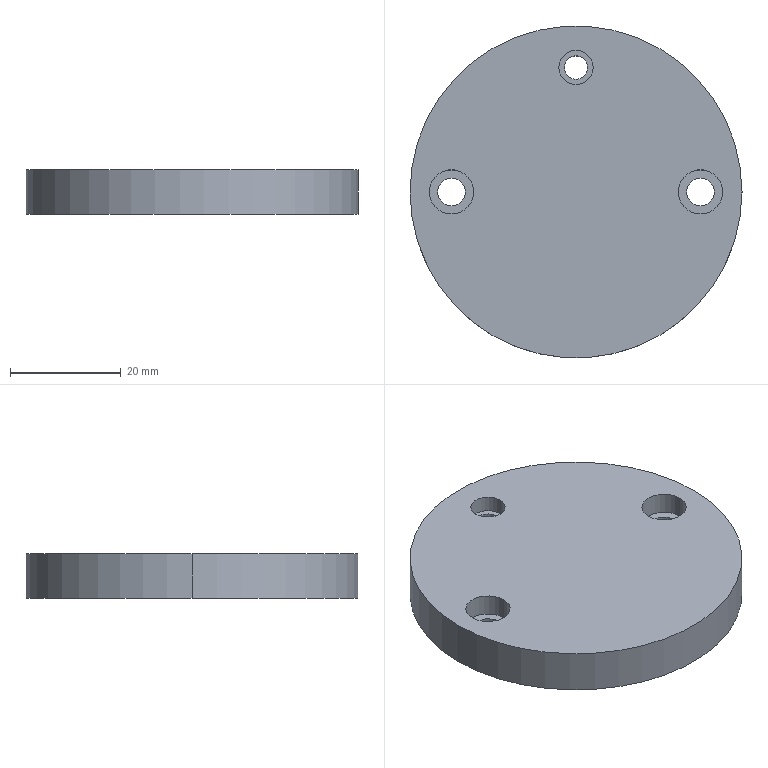Part | SolidWorks | features ICE 2, FlatPattern 1, SMBaseFlange 1, SheetMetal 1 | 1 solid | 19 faces | box 60 x 60 x 8 mm | volume 21900 mm3 | cylinder 14 | plane 5 | commonest cylinder face diameters 5 x4 8 x4 4.2 x2 6.2 x2 60 x2
STEP:
#1=CARTESIAN_POINT('',(1109.415,222.492,-3.));
#2=VERTEX_POINT('',#1);
#3=CARTESIAN_POINT('',(1115.615,222.492,-3.));
#4=VERTEX_POINT('',#3);
#5=CARTESIAN_POINT('',(1112.515,222.492,-3.));
#6=DIRECTION('',(0.,0.,1.));
#7=DIRECTION('',(1.,0.,0.));
#8=AXIS2_PLACEMENT_3D('',#5,#6,#7);
#9=CIRCLE('',#8,3.1);
#10=EDGE_CURVE('',#2,#4,#9,.T.);
#11=ORIENTED_EDGE('',*,*,#10,.F.);
#12=CARTESIAN_POINT('',(1109.415,222.492,0.));
#13=VERTEX_POINT('',#12);
#14=CARTESIAN_POINT('',(1109.415,222.492,-3.));
#15=DIRECTION('',(0.,0.,1.));
#16=VECTOR('',#15,1000.);
#17=LINE('',#14,#16);
#18=EDGE_CURVE('',#2,#13,#17,.T.);
#19=ORIENTED_EDGE('',*,*,#18,.T.);
#20=CARTESIAN_POINT('',(1115.615,222.492,0.));
#21=VERTEX_POINT('',#20);
#22=CARTESIAN_POINT('',(1112.515,222.492,0.));
#23=DIRECTION('',(0.,0.,1.));
#24=DIRECTION('',(1.,0.,0.));
#25=AXIS2_PLACEMENT_3D('',#22,#23,#24);
#26=CIRCLE('',#25,3.1);
#27=EDGE_CURVE('',#13,#21,#26,.T.);
#28=ORIENTED_EDGE('',*,*,#27,.T.);
#29=CARTESIAN_POINT('',(1115.615,222.492,-3.));
#30=DIRECTION('',(0.,0.,1.));
#31=VECTOR('',#30,1000.);
#32=LINE('',#29,#31);
#33=EDGE_CURVE('',#4,#21,#32,.T.);
#34=ORIENTED_EDGE('',*,*,#33,.F.);
#35=EDGE_LOOP('',(#11,#19,#28,#34));
#36=FACE_OUTER_BOUND('',#35,.T.);
#37=CARTESIAN_POINT('',(1112.515,222.492,-3.));
#38=DIRECTION('',(0.,0.,1.));
#39=DIRECTION('',(1.,0.,0.));
#40=AXIS2_PLACEMENT_3D('',#37,#38,#39);
#41=CYLINDRICAL_SURFACE('',#40,3.1);
#42=ADVANCED_FACE('',(#36),#41,.F.);
#43=CARTESIAN_POINT('',(1131.015,199.992,-4.));
#44=VERTEX_POINT('',#43);
#45=CARTESIAN_POINT('',(1139.015,199.992,-4.));
#46=VERTEX_POINT('',#45);
#47=CARTESIAN_POINT('',(1135.015,199.992,-4.));
#48=DIRECTION('',(0.,0.,1.));
#49=DIRECTION('',(1.,0.,0.));
#50=AXIS2_PLACEMENT_3D('',#47,#48,#49);
#51=CIRCLE('',#50,4.);
#52=EDGE_CURVE('',#44,#46,#51,.T.);
#53=ORIENTED_EDGE('',*,*,#52,.F.);
#54=CARTESIAN_POINT('',(1131.015,199.992,0.));
#55=VERTEX_POINT('',#54);
#56=CARTESIAN_POINT('',(1131.015,199.992,-4.));
#57=DIRECTION('',(0.,0.,1.));
#58=VECTOR('',#57,1000.);
#59=LINE('',#56,#58);
#60=EDGE_CURVE('',#44,#55,#59,.T.);
#61=ORIENTED_EDGE('',*,*,#60,.T.);
#62=CARTESIAN_POINT('',(1139.015,199.992,0.));
#63=VERTEX_POINT('',#62);
#64=CARTESIAN_POINT('',(1135.015,199.992,0.));
#65=DIRECTION('',(0.,0.,1.));
#66=DIRECTION('',(1.,0.,0.));
#67=AXIS2_PLACEMENT_3D('',#64,#65,#66);
#68=CIRCLE('',#67,4.);
#69=EDGE_CURVE('',#55,#63,#68,.T.);
#70=ORIENTED_EDGE('',*,*,#69,.T.);
#71=CARTESIAN_POINT('',(1139.015,199.992,-4.));
#72=DIRECTION('',(0.,0.,1.));
#73=VECTOR('',#72,1000.);
#74=LINE('',#71,#73);
#75=EDGE_CURVE('',#46,#63,#74,.T.);
#76=ORIENTED_EDGE('',*,*,#75,.F.);
#77=EDGE_LOOP('',(#53,#61,#70,#76));
#78=FACE_OUTER_BOUND('',#77,.T.);
#79=CARTESIAN_POINT('',(1135.015,199.992,-4.));
#80=DIRECTION('',(0.,0.,1.));
#81=DIRECTION('',(1.,0.,0.));
#82=AXIS2_PLACEMENT_3D('',#79,#80,#81);
#83=CYLINDRICAL_SURFACE('',#82,4.);
#84=ADVANCED_FACE('',(#78),#83,.F.);
#85=CARTESIAN_POINT('',(1086.015,199.992,-4.));
#86=VERTEX_POINT('',#85);
#87=CARTESIAN_POINT('',(1094.015,199.992,-4.));
#88=VERTEX_POINT('',#87);
#89=CARTESIAN_POINT('',(1090.015,199.992,-4.));
#90=DIRECTION('',(0.,0.,1.));
#91=DIRECTION('',(1.,0.,0.));
#92=AXIS2_PLACEMENT_3D('',#89,#90,#91);
#93=CIRCLE('',#92,4.);
#94=EDGE_CURVE('',#86,#88,#93,.T.);
#95=ORIENTED_EDGE('',*,*,#94,.F.);
#96=CARTESIAN_POINT('',(1086.015,199.992,0.));
#97=VERTEX_POINT('',#96);
#98=CARTESIAN_POINT('',(1086.015,199.992,-4.));
#99=DIRECTION('',(0.,0.,1.));
#100=VECTOR('',#99,1000.);
#101=LINE('',#98,#100);
#102=EDGE_CURVE('',#86,#97,#101,.T.);
#103=ORIENTED_EDGE('',*,*,#102,.T.);
#104=CARTESIAN_POINT('',(1094.015,199.992,0.));
#105=VERTEX_POINT('',#104);
#106=CARTESIAN_POINT('',(1090.015,199.992,0.));
#107=DIRECTION('',(0.,0.,1.));
#108=DIRECTION('',(1.,0.,0.));
#109=AXIS2_PLACEMENT_3D('',#106,#107,#108);
#110=CIRCLE('',#109,4.);
#111=EDGE_CURVE('',#97,#105,#110,.T.);
#112=ORIENTED_EDGE('',*,*,#111,.T.);
#113=CARTESIAN_POINT('',(1094.015,199.992,-4.));
#114=DIRECTION('',(0.,0.,1.));
#115=VECTOR('',#114,1000.);
#116=LINE('',#113,#115);
#117=EDGE_CURVE('',#88,#105,#116,.T.);
#118=ORIENTED_EDGE('',*,*,#117,.F.);
#119=EDGE_LOOP('',(#95,#103,#112,#118));
#120=FACE_OUTER_BOUND('',#119,.T.);
#121=CARTESIAN_POINT('',(1090.015,199.992,-4.));
#122=DIRECTION('',(0.,0.,1.));
#123=DIRECTION('',(1.,0.,0.));
#124=AXIS2_PLACEMENT_3D('',#121,#122,#123);
#125=CYLINDRICAL_SURFACE('',#124,4.);
#126=ADVANCED_FACE('',(#120),#125,.F.);
#127=CARTESIAN_POINT('',(1142.515,199.992,-8.));
#128=VERTEX_POINT('',#127);
#129=CARTESIAN_POINT('',(1082.515,199.992,-8.));
#130=VERTEX_POINT('',#129);
#131=CARTESIAN_POINT('',(1112.515,199.992,-8.));
#132=DIRECTION('',(0.,0.,1.));
#133=DIRECTION('',(1.,0.,0.));
#134=AXIS2_PLACEMENT_3D('',#131,#132,#133);
#135=CIRCLE('',#134,30.);
#136=EDGE_CURVE('',#128,#130,#135,.T.);
#137=ORIENTED_EDGE('',*,*,#136,.T.);
#138=CARTESIAN_POINT('',(1082.515,199.992,0.));
#139=VERTEX_POINT('',#138);
#140=CARTESIAN_POINT('',(1082.515,199.992,-8.));
#141=DIRECTION('',(0.,0.,1.));
#142=VECTOR('',#141,1000.);
#143=LINE('',#140,#142);
#144=EDGE_CURVE('',#130,#139,#143,.T.);
#145=ORIENTED_EDGE('',*,*,#144,.T.);
#146=CARTESIAN_POINT('',(1142.515,199.992,0.));
#147=VERTEX_POINT('',#146);
#148=CARTESIAN_POINT('',(1112.515,199.992,0.));
#149=DIRECTION('',(0.,0.,1.));
#150=DIRECTION('',(1.,0.,0.));
#151=AXIS2_PLACEMENT_3D('',#148,#149,#150);
#152=CIRCLE('',#151,30.);
#153=EDGE_CURVE('',#147,#139,#152,.T.);
#154=ORIENTED_EDGE('',*,*,#153,.F.);
#155=CARTESIAN_POINT('',(1142.515,199.992,-8.));
#156=DIRECTION('',(0.,0.,1.));
#157=VECTOR('',#156,1000.);
#158=LINE('',#155,#157);
#159=EDGE_CURVE('',#128,#147,#158,.T.);
#160=ORIENTED_EDGE('',*,*,#159,.F.);
#161=EDGE_LOOP('',(#137,#145,#154,#160));
#162=FACE_OUTER_BOUND('',#161,.T.);
#163=CARTESIAN_POINT('',(1112.515,199.992,-8.));
#164=DIRECTION('',(0.,0.,1.));
#165=DIRECTION('',(1.,0.,0.));
#166=AXIS2_PLACEMENT_3D('',#163,#164,#165);
#167=CYLINDRICAL_SURFACE('',#166,30.);
#168=ADVANCED_FACE('',(#162),#167,.T.);
#169=CARTESIAN_POINT('',(1087.515,199.992,-8.));
#170=VERTEX_POINT('',#169);
#171=CARTESIAN_POINT('',(1092.515,199.992,-8.));
#172=VERTEX_POINT('',#171);
#173=CARTESIAN_POINT('',(1090.015,199.992,-8.));
#174=DIRECTION('',(0.,0.,1.));
#175=DIRECTION('',(1.,0.,0.));
#176=AXIS2_PLACEMENT_3D('',#173,#174,#175);
#177=CIRCLE('',#176,2.5);
#178=EDGE_CURVE('',#170,#172,#177,.T.);
#179=ORIENTED_EDGE('',*,*,#178,.F.);
#180=CARTESIAN_POINT('',(1087.515,199.992,-4.));
#181=VERTEX_POINT('',#180);
#182=CARTESIAN_POINT('',(1087.515,199.992,-8.));
#183=DIRECTION('',(0.,0.,1.));
#184=VECTOR('',#183,1000.);
#185=LINE('',#182,#184);
#186=EDGE_CURVE('',#170,#181,#185,.T.);
#187=ORIENTED_EDGE('',*,*,#186,.T.);
#188=CARTESIAN_POINT('',(1092.515,199.992,-4.));
#189=VERTEX_POINT('',#188);
#190=CARTESIAN_POINT('',(1090.015,199.992,-4.));
#191=DIRECTION('',(0.,0.,-1.));
#192=DIRECTION('',(1.,0.,0.));
#193=AXIS2_PLACEMENT_3D('',#190,#191,#192);
#194=CIRCLE('',#193,2.5);
#195=EDGE_CURVE('',#189,#181,#194,.T.);
#196=ORIENTED_EDGE('',*,*,#195,.F.);
#197=CARTESIAN_POINT('',(1092.515,199.992,-8.));
#198=DIRECTION('',(0.,0.,1.));
#199=VECTOR('',#198,1000.);
#200=LINE('',#197,#199);
#201=EDGE_CURVE('',#172,#189,#200,.T.);
#202=ORIENTED_EDGE('',*,*,#201,.F.);
#203=EDGE_LOOP('',(#179,#187,#196,#202));
#204=FACE_OUTER_BOUND('',#203,.T.);
#205=CARTESIAN_POINT('',(1090.015,199.992,-8.));
#206=DIRECTION('',(0.,0.,1.));
#207=DIRECTION('',(1.,0.,0.));
#208=AXIS2_PLACEMENT_3D('',#205,#206,#207);
#209=CYLINDRICAL_SURFACE('',#208,2.5);
#210=ADVANCED_FACE('',(#204),#209,.F.);
#211=CARTESIAN_POINT('',(1132.515,199.992,-8.));
#212=VERTEX_POINT('',#211);
#213=CARTESIAN_POINT('',(1137.515,199.992,-8.));
#214=VERTEX_POINT('',#213);
#215=CARTESIAN_POINT('',(1135.015,199.992,-8.));
#216=DIRECTION('',(0.,0.,1.));
#217=DIRECTION('',(1.,0.,0.));
#218=AXIS2_PLACEMENT_3D('',#215,#216,#217);
#219=CIRCLE('',#218,2.5);
#220=EDGE_CURVE('',#212,#214,#219,.T.);
#221=ORIENTED_EDGE('',*,*,#220,.F.);
#222=CARTESIAN_POINT('',(1132.515,199.992,-4.));
#223=VERTEX_POINT('',#222);
#224=CARTESIAN_POINT('',(1132.515,199.992,-8.));
#225=DIRECTION('',(0.,0.,1.));
#226=VECTOR('',#225,1000.);
#227=LINE('',#224,#226);
#228=EDGE_CURVE('',#212,#223,#227,.T.);
#229=ORIENTED_EDGE('',*,*,#228,.T.);
#230=CARTESIAN_POINT('',(1137.515,199.992,-4.));
#231=VERTEX_POINT('',#230);
#232=CARTESIAN_POINT('',(1135.015,199.992,-4.));
#233=DIRECTION('',(0.,0.,-1.));
#234=DIRECTION('',(1.,0.,0.));
#235=AXIS2_PLACEMENT_3D('',#232,#233,#234);
#236=CIRCLE('',#235,2.5);
#237=EDGE_CURVE('',#231,#223,#236,.T.);
#238=ORIENTED_EDGE('',*,*,#237,.F.);
#239=CARTESIAN_POINT('',(1137.515,199.992,-8.));
#240=DIRECTION('',(0.,0.,1.));
#241=VECTOR('',#240,1000.);
#242=LINE('',#239,#241);
#243=EDGE_CURVE('',#214,#231,#242,.T.);
#244=ORIENTED_EDGE('',*,*,#243,.F.);
#245=EDGE_LOOP('',(#221,#229,#238,#244));
#246=FACE_OUTER_BOUND('',#245,.T.);
#247=CARTESIAN_POINT('',(1135.015,199.992,-8.));
#248=DIRECTION('',(0.,0.,1.));
#249=DIRECTION('',(1.,0.,0.));
#250=AXIS2_PLACEMENT_3D('',#247,#248,#249);
#251=CYLINDRICAL_SURFACE('',#250,2.5);
#252=ADVANCED_FACE('',(#246),#251,.F.);
#253=CARTESIAN_POINT('',(1110.415,222.492,-8.));
#254=VERTEX_POINT('',#253);
#255=CARTESIAN_POINT('',(1114.615,222.492,-8.));
#256=VERTEX_POINT('',#255);
#257=CARTESIAN_POINT('',(1112.515,222.492,-8.));
#258=DIRECTION('',(0.,0.,1.));
#259=DIRECTION('',(1.,0.,0.));
#260=AXIS2_PLACEMENT_3D('',#257,#258,#259);
#261=CIRCLE('',#260,2.1);
#262=EDGE_CURVE('',#254,#256,#261,.T.);
#263=ORIENTED_EDGE('',*,*,#262,.F.);
#264=CARTESIAN_POINT('',(1110.415,222.492,-3.));
#265=VERTEX_POINT('',#264);
#266=CARTESIAN_POINT('',(1110.415,222.492,-8.));
#267=DIRECTION('',(0.,0.,1.));
#268=VECTOR('',#267,1000.);
#269=LINE('',#266,#268);
#270=EDGE_CURVE('',#254,#265,#269,.T.);
#271=ORIENTED_EDGE('',*,*,#270,.T.);
#272=CARTESIAN_POINT('',(1114.615,222.492,-3.));
#273=VERTEX_POINT('',#272);
#274=CARTESIAN_POINT('',(1112.515,222.492,-3.));
#275=DIRECTION('',(0.,0.,-1.));
#276=DIRECTION('',(1.,0.,0.));
#277=AXIS2_PLACEMENT_3D('',#274,#275,#276);
#278=CIRCLE('',#277,2.1);
#279=EDGE_CURVE('',#273,#265,#278,.T.);
#280=ORIENTED_EDGE('',*,*,#279,.F.);
#281=CARTESIAN_POINT('',(1114.615,222.492,-8.));
#282=DIRECTION('',(0.,0.,1.));
#283=VECTOR('',#282,1000.);
#284=LINE('',#281,#283);
#285=EDGE_CURVE('',#256,#273,#284,.T.);
#286=ORIENTED_EDGE('',*,*,#285,.F.);
#287=EDGE_LOOP('',(#263,#271,#280,#286));
#288=FACE_OUTER_BOUND('',#287,.T.);
#289=CARTESIAN_POINT('',(1112.515,222.492,-8.));
#290=DIRECTION('',(0.,0.,1.));
#291=DIRECTION('',(1.,0.,0.));
#292=AXIS2_PLACEMENT_3D('',#289,#290,#291);
#293=CYLINDRICAL_SURFACE('',#292,2.1);
#294=ADVANCED_FACE('',(#288),#293,.F.);
#295=ORIENTED_EDGE('',*,*,#270,.F.);
#296=CARTESIAN_POINT('',(1112.515,222.492,-8.));
#297=DIRECTION('',(0.,0.,1.));
#298=DIRECTION('',(1.,0.,0.));
#299=AXIS2_PLACEMENT_3D('',#296,#297,#298);
#300=CIRCLE('',#299,2.1);
#301=EDGE_CURVE('',#256,#254,#300,.T.);
#302=ORIENTED_EDGE('',*,*,#301,.F.);
#303=ORIENTED_EDGE('',*,*,#285,.T.);
#304=CARTESIAN_POINT('',(1112.515,222.492,-3.));
#305=DIRECTION('',(0.,0.,-1.));
#306=DIRECTION('',(1.,0.,0.));
#307=AXIS2_PLACEMENT_3D('',#304,#305,#306);
#308=CIRCLE('',#307,2.1);
#309=EDGE_CURVE('',#265,#273,#308,.T.);
#310=ORIENTED_EDGE('',*,*,#309,.F.);
#311=EDGE_LOOP('',(#295,#302,#303,#310));
#312=FACE_OUTER_BOUND('',#311,.T.);
#313=CARTESIAN_POINT('',(1112.515,222.492,-8.));
#314=DIRECTION('',(0.,0.,1.));
#315=DIRECTION('',(1.,0.,0.));
#316=AXIS2_PLACEMENT_3D('',#313,#314,#315);
#317=CYLINDRICAL_SURFACE('',#316,2.1);
#318=ADVANCED_FACE('',(#312),#317,.F.);
#319=ORIENTED_EDGE('',*,*,#228,.F.);
#320=CARTESIAN_POINT('',(1135.015,199.992,-8.));
#321=DIRECTION('',(0.,0.,1.));
#322=DIRECTION('',(1.,0.,0.));
#323=AXIS2_PLACEMENT_3D('',#320,#321,#322);
#324=CIRCLE('',#323,2.5);
#325=EDGE_CURVE('',#214,#212,#324,.T.);
#326=ORIENTED_EDGE('',*,*,#325,.F.);
#327=ORIENTED_EDGE('',*,*,#243,.T.);
#328=CARTESIAN_POINT('',(1135.015,199.992,-4.));
#329=DIRECTION('',(0.,0.,-1.));
#330=DIRECTION('',(1.,0.,0.));
#331=AXIS2_PLACEMENT_3D('',#328,#329,#330);
#332=CIRCLE('',#331,2.5);
#333=EDGE_CURVE('',#223,#231,#332,.T.);
#334=ORIENTED_EDGE('',*,*,#333,.F.);
#335=EDGE_LOOP('',(#319,#326,#327,#334));
#336=FACE_OUTER_BOUND('',#335,.T.);
#337=CARTESIAN_POINT('',(1135.015,199.992,-8.));
#338=DIRECTION('',(0.,0.,1.));
#339=DIRECTION('',(1.,0.,0.));
#340=AXIS2_PLACEMENT_3D('',#337,#338,#339);
#341=CYLINDRICAL_SURFACE('',#340,2.5);
#342=ADVANCED_FACE('',(#336),#341,.F.);
#343=ORIENTED_EDGE('',*,*,#186,.F.);
#344=CARTESIAN_POINT('',(1090.015,199.992,-8.));
#345=DIRECTION('',(0.,0.,1.));
#346=DIRECTION('',(1.,0.,0.));
#347=AXIS2_PLACEMENT_3D('',#344,#345,#346);
#348=CIRCLE('',#347,2.5);
#349=EDGE_CURVE('',#172,#170,#348,.T.);
#350=ORIENTED_EDGE('',*,*,#349,.F.);
#351=ORIENTED_EDGE('',*,*,#201,.T.);
#352=CARTESIAN_POINT('',(1090.015,199.992,-4.));
#353=DIRECTION('',(0.,0.,-1.));
#354=DIRECTION('',(1.,0.,0.));
#355=AXIS2_PLACEMENT_3D('',#352,#353,#354);
#356=CIRCLE('',#355,2.5);
#357=EDGE_CURVE('',#181,#189,#356,.T.);
#358=ORIENTED_EDGE('',*,*,#357,.F.);
#359=EDGE_LOOP('',(#343,#350,#351,#358));
#360=FACE_OUTER_BOUND('',#359,.T.);
#361=CARTESIAN_POINT('',(1090.015,199.992,-8.));
#362=DIRECTION('',(0.,0.,1.));
#363=DIRECTION('',(1.,0.,0.));
#364=AXIS2_PLACEMENT_3D('',#361,#362,#363);
#365=CYLINDRICAL_SURFACE('',#364,2.5);
#366=ADVANCED_FACE('',(#360),#365,.F.);
#367=ORIENTED_EDGE('',*,*,#144,.F.);
#368=CARTESIAN_POINT('',(1112.515,199.992,-8.));
#369=DIRECTION('',(0.,0.,1.));
#370=DIRECTION('',(1.,0.,0.));
#371=AXIS2_PLACEMENT_3D('',#368,#369,#370);
#372=CIRCLE('',#371,30.);
#373=EDGE_CURVE('',#130,#128,#372,.T.);
#374=ORIENTED_EDGE('',*,*,#373,.T.);
#375=ORIENTED_EDGE('',*,*,#159,.T.);
#376=CARTESIAN_POINT('',(1112.515,199.992,0.));
#377=DIRECTION('',(0.,0.,1.));
#378=DIRECTION('',(1.,0.,0.));
#379=AXIS2_PLACEMENT_3D('',#376,#377,#378);
#380=CIRCLE('',#379,30.);
#381=EDGE_CURVE('',#139,#147,#380,.T.);
#382=ORIENTED_EDGE('',*,*,#381,.F.);
#383=EDGE_LOOP('',(#367,#374,#375,#382));
#384=FACE_OUTER_BOUND('',#383,.T.);
#385=CARTESIAN_POINT('',(1112.515,199.992,-8.));
#386=DIRECTION('',(0.,0.,1.));
#387=DIRECTION('',(1.,0.,0.));
#388=AXIS2_PLACEMENT_3D('',#385,#386,#387);
#389=CYLINDRICAL_SURFACE('',#388,30.);
#390=ADVANCED_FACE('',(#384),#389,.T.);
#391=ORIENTED_EDGE('',*,*,#301,.T.);
#392=ORIENTED_EDGE('',*,*,#262,.T.);
#393=EDGE_LOOP('',(#391,#392));
#394=FACE_BOUND('',#393,.T.);
#395=ORIENTED_EDGE('',*,*,#349,.T.);
#396=ORIENTED_EDGE('',*,*,#178,.T.);
#397=EDGE_LOOP('',(#395,#396));
#398=FACE_BOUND('',#397,.T.);
#399=ORIENTED_EDGE('',*,*,#325,.T.);
#400=ORIENTED_EDGE('',*,*,#220,.T.);
#401=EDGE_LOOP('',(#399,#400));
#402=FACE_BOUND('',#401,.T.);
#403=ORIENTED_EDGE('',*,*,#136,.F.);
#404=ORIENTED_EDGE('',*,*,#373,.F.);
#405=EDGE_LOOP('',(#403,#404));
#406=FACE_OUTER_BOUND('',#405,.T.);
#407=CARTESIAN_POINT('',(1112.515,199.992,-8.));
#408=DIRECTION('',(0.,0.,1.));
#409=DIRECTION('',(1.,0.,0.));
#410=AXIS2_PLACEMENT_3D('',#407,#408,#409);
#411=PLANE('',#410);
#412=ADVANCED_FACE('',(#394,#398,#402,#406),#411,.F.);
#413=CARTESIAN_POINT('',(1112.515,222.492,0.));
#414=DIRECTION('',(0.,0.,1.));
#415=DIRECTION('',(1.,0.,0.));
#416=AXIS2_PLACEMENT_3D('',#413,#414,#415);
#417=CIRCLE('',#416,3.1);
#418=EDGE_CURVE('',#21,#13,#417,.T.);
#419=ORIENTED_EDGE('',*,*,#418,.F.);
#420=ORIENTED_EDGE('',*,*,#27,.F.);
#421=EDGE_LOOP('',(#419,#420));
#422=FACE_BOUND('',#421,.T.);
#423=CARTESIAN_POINT('',(1135.015,199.992,0.));
#424=DIRECTION('',(0.,0.,1.));
#425=DIRECTION('',(1.,0.,0.));
#426=AXIS2_PLACEMENT_3D('',#423,#424,#425);
#427=CIRCLE('',#426,4.);
#428=EDGE_CURVE('',#63,#55,#427,.T.);
#429=ORIENTED_EDGE('',*,*,#428,.F.);
#430=ORIENTED_EDGE('',*,*,#69,.F.);
#431=EDGE_LOOP('',(#429,#430));
#432=FACE_BOUND('',#431,.T.);
#433=CARTESIAN_POINT('',(1090.015,199.992,0.));
#434=DIRECTION('',(0.,0.,1.));
#435=DIRECTION('',(1.,0.,0.));
#436=AXIS2_PLACEMENT_3D('',#433,#434,#435);
#437=CIRCLE('',#436,4.);
#438=EDGE_CURVE('',#105,#97,#437,.T.);
#439=ORIENTED_EDGE('',*,*,#438,.F.);
#440=ORIENTED_EDGE('',*,*,#111,.F.);
#441=EDGE_LOOP('',(#439,#440));
#442=FACE_BOUND('',#441,.T.);
#443=ORIENTED_EDGE('',*,*,#153,.T.);
#444=ORIENTED_EDGE('',*,*,#381,.T.);
#445=EDGE_LOOP('',(#443,#444));
#446=FACE_OUTER_BOUND('',#445,.T.);
#447=CARTESIAN_POINT('',(1112.515,199.992,0.));
#448=DIRECTION('',(0.,0.,1.));
#449=DIRECTION('',(1.,0.,0.));
#450=AXIS2_PLACEMENT_3D('',#447,#448,#449);
#451=PLANE('',#450);
#452=ADVANCED_FACE('',(#422,#432,#442,#446),#451,.T.);
#453=CARTESIAN_POINT('',(1090.015,199.992,-4.));
#454=DIRECTION('',(0.,0.,1.));
#455=DIRECTION('',(1.,0.,0.));
#456=AXIS2_PLACEMENT_3D('',#453,#454,#455);
#457=CIRCLE('',#456,4.);
#458=EDGE_CURVE('',#88,#86,#457,.T.);
#459=ORIENTED_EDGE('',*,*,#458,.T.);
#460=ORIENTED_EDGE('',*,*,#94,.T.);
#461=EDGE_LOOP('',(#459,#460));
#462=FACE_OUTER_BOUND('',#461,.T.);
#463=ORIENTED_EDGE('',*,*,#195,.T.);
#464=ORIENTED_EDGE('',*,*,#357,.T.);
#465=EDGE_LOOP('',(#463,#464));
#466=FACE_BOUND('',#465,.T.);
#467=CARTESIAN_POINT('',(1090.015,199.992,-4.));
#468=DIRECTION('',(0.,0.,1.));
#469=DIRECTION('',(1.,0.,0.));
#470=AXIS2_PLACEMENT_3D('',#467,#468,#469);
#471=PLANE('',#470);
#472=ADVANCED_FACE('',(#462,#466),#471,.T.);
#473=ORIENTED_EDGE('',*,*,#102,.F.);
#474=ORIENTED_EDGE('',*,*,#458,.F.);
#475=ORIENTED_EDGE('',*,*,#117,.T.);
#476=ORIENTED_EDGE('',*,*,#438,.T.);
#477=EDGE_LOOP('',(#473,#474,#475,#476));
#478=FACE_OUTER_BOUND('',#477,.T.);
#479=CARTESIAN_POINT('',(1090.015,199.992,-4.));
#480=DIRECTION('',(0.,0.,1.));
#481=DIRECTION('',(1.,0.,0.));
#482=AXIS2_PLACEMENT_3D('',#479,#480,#481);
#483=CYLINDRICAL_SURFACE('',#482,4.);
#484=ADVANCED_FACE('',(#478),#483,.F.);
#485=CARTESIAN_POINT('',(1135.015,199.992,-4.));
#486=DIRECTION('',(0.,0.,1.));
#487=DIRECTION('',(1.,0.,0.));
#488=AXIS2_PLACEMENT_3D('',#485,#486,#487);
#489=CIRCLE('',#488,4.);
#490=EDGE_CURVE('',#46,#44,#489,.T.);
#491=ORIENTED_EDGE('',*,*,#490,.T.);
#492=ORIENTED_EDGE('',*,*,#52,.T.);
#493=EDGE_LOOP('',(#491,#492));
#494=FACE_OUTER_BOUND('',#493,.T.);
#495=ORIENTED_EDGE('',*,*,#237,.T.);
#496=ORIENTED_EDGE('',*,*,#333,.T.);
#497=EDGE_LOOP('',(#495,#496));
#498=FACE_BOUND('',#497,.T.);
#499=CARTESIAN_POINT('',(1135.015,199.992,-4.));
#500=DIRECTION('',(0.,0.,1.));
#501=DIRECTION('',(1.,0.,0.));
#502=AXIS2_PLACEMENT_3D('',#499,#500,#501);
#503=PLANE('',#502);
#504=ADVANCED_FACE('',(#494,#498),#503,.T.);
#505=ORIENTED_EDGE('',*,*,#60,.F.);
#506=ORIENTED_EDGE('',*,*,#490,.F.);
#507=ORIENTED_EDGE('',*,*,#75,.T.);
#508=ORIENTED_EDGE('',*,*,#428,.T.);
#509=EDGE_LOOP('',(#505,#506,#507,#508));
#510=FACE_OUTER_BOUND('',#509,.T.);
#511=CARTESIAN_POINT('',(1135.015,199.992,-4.));
#512=DIRECTION('',(0.,0.,1.));
#513=DIRECTION('',(1.,0.,0.));
#514=AXIS2_PLACEMENT_3D('',#511,#512,#513);
#515=CYLINDRICAL_SURFACE('',#514,4.);
#516=ADVANCED_FACE('',(#510),#515,.F.);
#517=CARTESIAN_POINT('',(1112.515,222.492,-3.));
#518=DIRECTION('',(0.,0.,1.));
#519=DIRECTION('',(1.,0.,0.));
#520=AXIS2_PLACEMENT_3D('',#517,#518,#519);
#521=CIRCLE('',#520,3.1);
#522=EDGE_CURVE('',#4,#2,#521,.T.);
#523=ORIENTED_EDGE('',*,*,#522,.T.);
#524=ORIENTED_EDGE('',*,*,#10,.T.);
#525=EDGE_LOOP('',(#523,#524));
#526=FACE_OUTER_BOUND('',#525,.T.);
#527=ORIENTED_EDGE('',*,*,#279,.T.);
#528=ORIENTED_EDGE('',*,*,#309,.T.);
#529=EDGE_LOOP('',(#527,#528));
#530=FACE_BOUND('',#529,.T.);
#531=CARTESIAN_POINT('',(1112.515,222.492,-3.));
#532=DIRECTION('',(0.,0.,1.));
#533=DIRECTION('',(1.,0.,0.));
#534=AXIS2_PLACEMENT_3D('',#531,#532,#533);
#535=PLANE('',#534);
#536=ADVANCED_FACE('',(#526,#530),#535,.T.);
#537=ORIENTED_EDGE('',*,*,#18,.F.);
#538=ORIENTED_EDGE('',*,*,#522,.F.);
#539=ORIENTED_EDGE('',*,*,#33,.T.);
#540=ORIENTED_EDGE('',*,*,#418,.T.);
#541=EDGE_LOOP('',(#537,#538,#539,#540));
#542=FACE_OUTER_BOUND('',#541,.T.);
#543=CARTESIAN_POINT('',(1112.515,222.492,-3.));
#544=DIRECTION('',(0.,0.,1.));
#545=DIRECTION('',(1.,0.,0.));
#546=AXIS2_PLACEMENT_3D('',#543,#544,#545);
#547=CYLINDRICAL_SURFACE('',#546,3.1);
#548=ADVANCED_FACE('',(#542),#547,.F.);
#549=CLOSED_SHELL('',(#42,#84,#126,#168,#210,#252,#294,#318,#342,#366,#390,#412,#452,#472,#484,#504,#516,#536,#548));
#550=MANIFOLD_SOLID_BREP('',#549);
#551=CARTESIAN_POINT('',(0.,0.,0.));
#552=DIRECTION('',(0.,0.,1.));
#553=DIRECTION('',(1.,0.,0.));
#554=AXIS2_PLACEMENT_3D('',#551,#552,#553);
#555=(LENGTH_UNIT()NAMED_UNIT(*)SI_UNIT(.MILLI.,.METRE.));
#556=UNCERTAINTY_MEASURE_WITH_UNIT(LENGTH_MEASURE(0.00001),#555,'','');
#557=(NAMED_UNIT(*)PLANE_ANGLE_UNIT()SI_UNIT($,.RADIAN.));
#558=(NAMED_UNIT(*)SI_UNIT($,.STERADIAN.)SOLID_ANGLE_UNIT());
#559=(GEOMETRIC_REPRESENTATION_CONTEXT(3)GLOBAL_UNCERTAINTY_ASSIGNED_CONTEXT((#556))GLOBAL_UNIT_ASSIGNED_CONTEXT((#555,#557,#558))REPRESENTATION_CONTEXT('',''));
#560=ADVANCED_BREP_SHAPE_REPRESENTATION('',(#550,#554),#559);